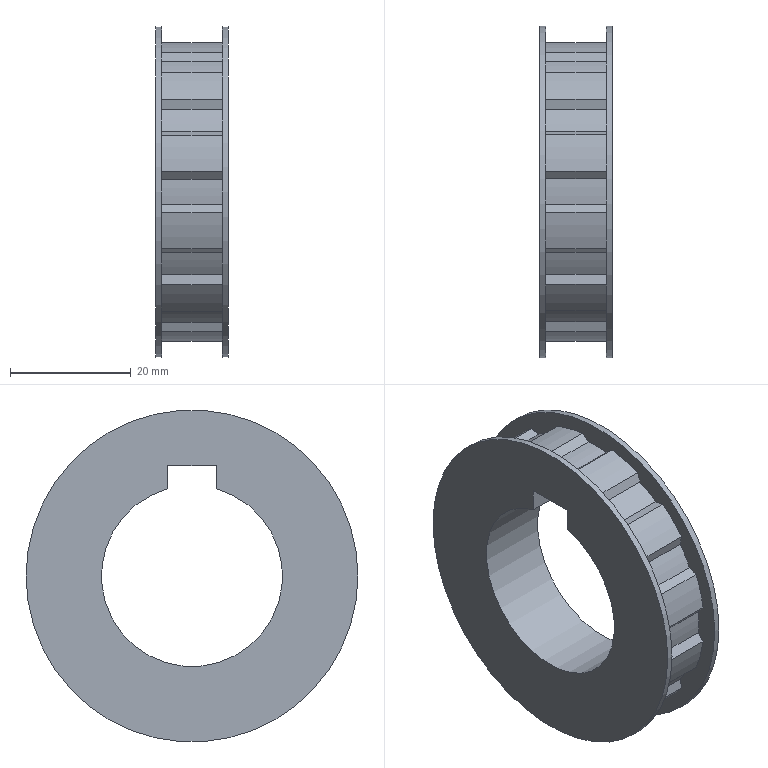Part | NX | features DATUM_CSYS 4, EXTRUDE 3, SKETCH 3, Container 1, EXTRACT_BODY 1, Geometry Instance 1, UNITE 1 | 1 solid | 58 faces | box 12 x 55 x 55 mm | volume 14742 mm3 | plane 31 | cylinder 27 | commonest cylinder face diameters 47.525 x12 50 x12 55 x2 30 x1